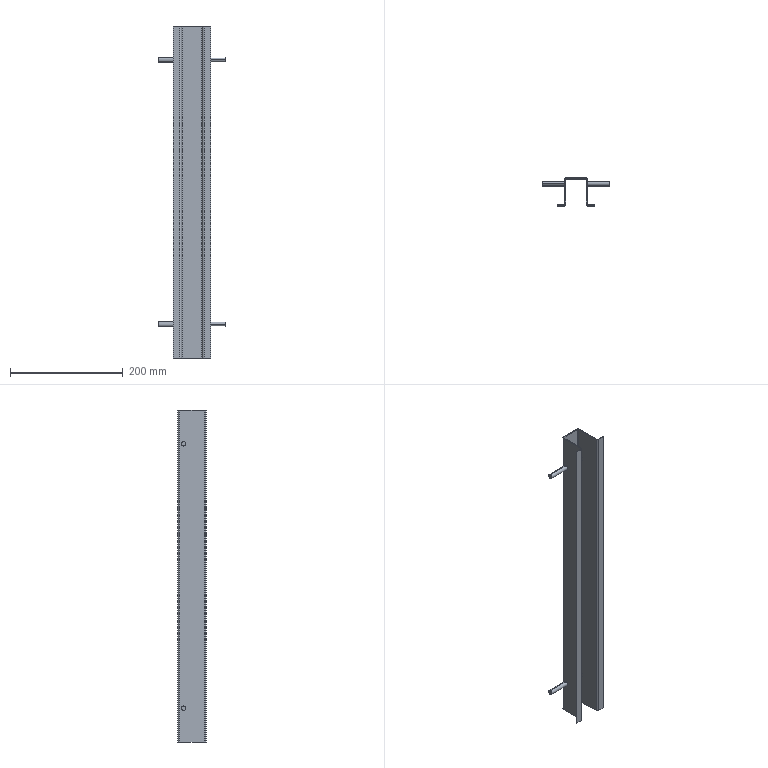Part | SolidWorks | features ICE 2, EdgeFlange 1, FlatPattern 1, SMBaseFlange 1, SheetMetal 1 | 1 solid | 50 faces | box 120 x 50 x 590 mm | volume 149764 mm3 | plane 34 | cylinder 16 | commonest cylinder face diameters 8 x8 3 x4 6 x4
STEP:
#1=CARTESIAN_POINT('',(-58.139,-0.4097,534.));
#2=VERTEX_POINT('',#1);
#3=CARTESIAN_POINT('',(-58.139,-0.4097,526.));
#4=VERTEX_POINT('',#3);
#5=CARTESIAN_POINT('',(-58.139,-0.4097,530.));
#6=DIRECTION('',(-1.,0.,0.));
#7=DIRECTION('',(0.,0.,1.));
#8=AXIS2_PLACEMENT_3D('',#5,#6,#7);
#9=CIRCLE('',#8,4.);
#10=EDGE_CURVE('',#2,#4,#9,.T.);
#11=ORIENTED_EDGE('',*,*,#10,.F.);
#12=CARTESIAN_POINT('',(-18.139,-0.4097,534.));
#13=VERTEX_POINT('',#12);
#14=CARTESIAN_POINT('',(-58.139,-0.4097,534.));
#15=DIRECTION('',(1.,0.,0.));
#16=VECTOR('',#15,1000.);
#17=LINE('',#14,#16);
#18=EDGE_CURVE('',#2,#13,#17,.T.);
#19=ORIENTED_EDGE('',*,*,#18,.T.);
#20=CARTESIAN_POINT('',(-18.139,-0.4097,526.));
#21=VERTEX_POINT('',#20);
#22=CARTESIAN_POINT('',(-18.139,-0.4097,530.));
#23=DIRECTION('',(-1.,0.,0.));
#24=DIRECTION('',(0.,0.,1.));
#25=AXIS2_PLACEMENT_3D('',#22,#23,#24);
#26=CIRCLE('',#25,4.);
#27=EDGE_CURVE('',#13,#21,#26,.T.);
#28=ORIENTED_EDGE('',*,*,#27,.T.);
#29=CARTESIAN_POINT('',(-58.139,-0.4097,526.));
#30=DIRECTION('',(1.,0.,0.));
#31=VECTOR('',#30,1000.);
#32=LINE('',#29,#31);
#33=EDGE_CURVE('',#4,#21,#32,.T.);
#34=ORIENTED_EDGE('',*,*,#33,.F.);
#35=EDGE_LOOP('',(#11,#19,#28,#34));
#36=FACE_OUTER_BOUND('',#35,.T.);
#37=CARTESIAN_POINT('',(-58.139,-0.4097,530.));
#38=DIRECTION('',(1.,0.,0.));
#39=DIRECTION('',(0.,0.,-1.));
#40=AXIS2_PLACEMENT_3D('',#37,#38,#39);
#41=CYLINDRICAL_SURFACE('',#40,4.);
#42=ADVANCED_FACE('',(#36),#41,.T.);
#43=CARTESIAN_POINT('',(-58.139,-0.4097,64.));
#44=VERTEX_POINT('',#43);
#45=CARTESIAN_POINT('',(-58.139,-0.4097,56.));
#46=VERTEX_POINT('',#45);
#47=CARTESIAN_POINT('',(-58.139,-0.4097,60.));
#48=DIRECTION('',(-1.,0.,0.));
#49=DIRECTION('',(0.,0.,1.));
#50=AXIS2_PLACEMENT_3D('',#47,#48,#49);
#51=CIRCLE('',#50,4.);
#52=EDGE_CURVE('',#44,#46,#51,.T.);
#53=ORIENTED_EDGE('',*,*,#52,.F.);
#54=CARTESIAN_POINT('',(-18.139,-0.4097,64.));
#55=VERTEX_POINT('',#54);
#56=CARTESIAN_POINT('',(-58.139,-0.4097,64.));
#57=DIRECTION('',(1.,0.,0.));
#58=VECTOR('',#57,1000.);
#59=LINE('',#56,#58);
#60=EDGE_CURVE('',#44,#55,#59,.T.);
#61=ORIENTED_EDGE('',*,*,#60,.T.);
#62=CARTESIAN_POINT('',(-18.139,-0.4097,56.));
#63=VERTEX_POINT('',#62);
#64=CARTESIAN_POINT('',(-18.139,-0.4097,60.));
#65=DIRECTION('',(-1.,0.,0.));
#66=DIRECTION('',(0.,0.,1.));
#67=AXIS2_PLACEMENT_3D('',#64,#65,#66);
#68=CIRCLE('',#67,4.);
#69=EDGE_CURVE('',#55,#63,#68,.T.);
#70=ORIENTED_EDGE('',*,*,#69,.T.);
#71=CARTESIAN_POINT('',(-58.139,-0.4097,56.));
#72=DIRECTION('',(1.,0.,0.));
#73=VECTOR('',#72,1000.);
#74=LINE('',#71,#73);
#75=EDGE_CURVE('',#46,#63,#74,.T.);
#76=ORIENTED_EDGE('',*,*,#75,.F.);
#77=EDGE_LOOP('',(#53,#61,#70,#76));
#78=FACE_OUTER_BOUND('',#77,.T.);
#79=CARTESIAN_POINT('',(-58.139,-0.4097,60.));
#80=DIRECTION('',(1.,0.,0.));
#81=DIRECTION('',(0.,0.,-1.));
#82=AXIS2_PLACEMENT_3D('',#79,#80,#81);
#83=CYLINDRICAL_SURFACE('',#82,4.);
#84=ADVANCED_FACE('',(#78),#83,.T.);
#85=CARTESIAN_POINT('',(61.861,3.59,60.));
#86=VERTEX_POINT('',#85);
#87=CARTESIAN_POINT('',(61.861,-4.41,60.));
#88=VERTEX_POINT('',#87);
#89=CARTESIAN_POINT('',(61.861,-0.4097,60.));
#90=DIRECTION('',(1.,0.,0.));
#91=DIRECTION('',(0.,1.,0.));
#92=AXIS2_PLACEMENT_3D('',#89,#90,#91);
#93=CIRCLE('',#92,4.);
#94=EDGE_CURVE('',#86,#88,#93,.T.);
#95=ORIENTED_EDGE('',*,*,#94,.F.);
#96=CARTESIAN_POINT('',(21.861,3.59,60.));
#97=VERTEX_POINT('',#96);
#98=CARTESIAN_POINT('',(61.861,3.59,60.));
#99=DIRECTION('',(-1.,0.,0.));
#100=VECTOR('',#99,1000.);
#101=LINE('',#98,#100);
#102=EDGE_CURVE('',#86,#97,#101,.T.);
#103=ORIENTED_EDGE('',*,*,#102,.T.);
#104=CARTESIAN_POINT('',(21.861,-4.41,60.));
#105=VERTEX_POINT('',#104);
#106=CARTESIAN_POINT('',(21.861,-0.4097,60.));
#107=DIRECTION('',(1.,0.,0.));
#108=DIRECTION('',(0.,1.,0.));
#109=AXIS2_PLACEMENT_3D('',#106,#107,#108);
#110=CIRCLE('',#109,4.);
#111=EDGE_CURVE('',#97,#105,#110,.T.);
#112=ORIENTED_EDGE('',*,*,#111,.T.);
#113=CARTESIAN_POINT('',(61.861,-4.41,60.));
#114=DIRECTION('',(-1.,0.,0.));
#115=VECTOR('',#114,1000.);
#116=LINE('',#113,#115);
#117=EDGE_CURVE('',#88,#105,#116,.T.);
#118=ORIENTED_EDGE('',*,*,#117,.F.);
#119=EDGE_LOOP('',(#95,#103,#112,#118));
#120=FACE_OUTER_BOUND('',#119,.T.);
#121=CARTESIAN_POINT('',(61.861,-0.4097,60.));
#122=DIRECTION('',(-1.,0.,0.));
#123=DIRECTION('',(0.,-1.,0.));
#124=AXIS2_PLACEMENT_3D('',#121,#122,#123);
#125=CYLINDRICAL_SURFACE('',#124,4.);
#126=ADVANCED_FACE('',(#120),#125,.T.);
#127=CARTESIAN_POINT('',(61.861,3.59,530.));
#128=VERTEX_POINT('',#127);
#129=CARTESIAN_POINT('',(61.861,-4.41,530.));
#130=VERTEX_POINT('',#129);
#131=CARTESIAN_POINT('',(61.861,-0.4097,530.));
#132=DIRECTION('',(1.,0.,0.));
#133=DIRECTION('',(0.,1.,0.));
#134=AXIS2_PLACEMENT_3D('',#131,#132,#133);
#135=CIRCLE('',#134,4.);
#136=EDGE_CURVE('',#128,#130,#135,.T.);
#137=ORIENTED_EDGE('',*,*,#136,.F.);
#138=CARTESIAN_POINT('',(21.861,3.59,530.));
#139=VERTEX_POINT('',#138);
#140=CARTESIAN_POINT('',(61.861,3.59,530.));
#141=DIRECTION('',(-1.,0.,0.));
#142=VECTOR('',#141,1000.);
#143=LINE('',#140,#142);
#144=EDGE_CURVE('',#128,#139,#143,.T.);
#145=ORIENTED_EDGE('',*,*,#144,.T.);
#146=CARTESIAN_POINT('',(21.861,-4.41,530.));
#147=VERTEX_POINT('',#146);
#148=CARTESIAN_POINT('',(21.861,-0.4097,530.));
#149=DIRECTION('',(1.,0.,0.));
#150=DIRECTION('',(0.,1.,0.));
#151=AXIS2_PLACEMENT_3D('',#148,#149,#150);
#152=CIRCLE('',#151,4.);
#153=EDGE_CURVE('',#139,#147,#152,.T.);
#154=ORIENTED_EDGE('',*,*,#153,.T.);
#155=CARTESIAN_POINT('',(61.861,-4.41,530.));
#156=DIRECTION('',(-1.,0.,0.));
#157=VECTOR('',#156,1000.);
#158=LINE('',#155,#157);
#159=EDGE_CURVE('',#130,#147,#158,.T.);
#160=ORIENTED_EDGE('',*,*,#159,.F.);
#161=EDGE_LOOP('',(#137,#145,#154,#160));
#162=FACE_OUTER_BOUND('',#161,.T.);
#163=CARTESIAN_POINT('',(61.861,-0.4097,530.));
#164=DIRECTION('',(-1.,0.,0.));
#165=DIRECTION('',(0.,-1.,0.));
#166=AXIS2_PLACEMENT_3D('',#163,#164,#165);
#167=CYLINDRICAL_SURFACE('',#166,4.);
#168=ADVANCED_FACE('',(#162),#167,.T.);
#169=CARTESIAN_POINT('',(-18.139,-0.4097,60.));
#170=DIRECTION('',(-1.,0.,0.));
#171=DIRECTION('',(0.,0.,1.));
#172=AXIS2_PLACEMENT_3D('',#169,#170,#171);
#173=CIRCLE('',#172,4.);
#174=EDGE_CURVE('',#63,#55,#173,.T.);
#175=ORIENTED_EDGE('',*,*,#174,.F.);
#176=ORIENTED_EDGE('',*,*,#69,.F.);
#177=EDGE_LOOP('',(#175,#176));
#178=FACE_BOUND('',#177,.T.);
#179=CARTESIAN_POINT('',(-18.139,-37.41,0.));
#180=VERTEX_POINT('',#179);
#181=CARTESIAN_POINT('',(-18.139,6.59,0.));
#182=VERTEX_POINT('',#181);
#183=CARTESIAN_POINT('',(-18.139,-40.41,0.));
#184=DIRECTION('',(0.,1.,0.));
#185=VECTOR('',#184,1000.);
#186=LINE('',#183,#185);
#187=EDGE_CURVE('',#180,#182,#186,.T.);
#188=ORIENTED_EDGE('',*,*,#187,.F.);
#189=CARTESIAN_POINT('',(-18.139,-37.41,590.));
#190=VERTEX_POINT('',#189);
#191=CARTESIAN_POINT('',(-18.139,-37.41,590.));
#192=DIRECTION('',(0.,0.,-1.));
#193=VECTOR('',#192,1000.);
#194=LINE('',#191,#193);
#195=EDGE_CURVE('',#190,#180,#194,.T.);
#196=ORIENTED_EDGE('',*,*,#195,.F.);
#197=CARTESIAN_POINT('',(-18.139,6.59,590.));
#198=VERTEX_POINT('',#197);
#199=CARTESIAN_POINT('',(-18.139,-40.41,590.));
#200=DIRECTION('',(0.,1.,0.));
#201=VECTOR('',#200,1000.);
#202=LINE('',#199,#201);
#203=EDGE_CURVE('',#190,#198,#202,.T.);
#204=ORIENTED_EDGE('',*,*,#203,.T.);
#205=CARTESIAN_POINT('',(-18.139,6.59,590.));
#206=DIRECTION('',(0.,0.,-1.));
#207=VECTOR('',#206,1000.);
#208=LINE('',#205,#207);
#209=EDGE_CURVE('',#198,#182,#208,.T.);
#210=ORIENTED_EDGE('',*,*,#209,.T.);
#211=EDGE_LOOP('',(#188,#196,#204,#210));
#212=FACE_OUTER_BOUND('',#211,.T.);
#213=CARTESIAN_POINT('',(-18.139,-0.4097,530.));
#214=DIRECTION('',(-1.,0.,0.));
#215=DIRECTION('',(0.,0.,1.));
#216=AXIS2_PLACEMENT_3D('',#213,#214,#215);
#217=CIRCLE('',#216,4.);
#218=EDGE_CURVE('',#21,#13,#217,.T.);
#219=ORIENTED_EDGE('',*,*,#218,.F.);
#220=ORIENTED_EDGE('',*,*,#27,.F.);
#221=EDGE_LOOP('',(#219,#220));
#222=FACE_BOUND('',#221,.T.);
#223=CARTESIAN_POINT('',(-18.139,-40.41,590.));
#224=DIRECTION('',(-1.,0.,0.));
#225=DIRECTION('',(0.,0.,1.));
#226=AXIS2_PLACEMENT_3D('',#223,#224,#225);
#227=PLANE('',#226);
#228=ADVANCED_FACE('',(#178,#212,#222),#227,.T.);
#229=CARTESIAN_POINT('',(21.861,-0.4097,530.));
#230=DIRECTION('',(1.,0.,0.));
#231=DIRECTION('',(0.,1.,0.));
#232=AXIS2_PLACEMENT_3D('',#229,#230,#231);
#233=CIRCLE('',#232,4.);
#234=EDGE_CURVE('',#147,#139,#233,.T.);
#235=ORIENTED_EDGE('',*,*,#234,.F.);
#236=ORIENTED_EDGE('',*,*,#153,.F.);
#237=EDGE_LOOP('',(#235,#236));
#238=FACE_BOUND('',#237,.T.);
#239=CARTESIAN_POINT('',(21.861,6.59,590.));
#240=VERTEX_POINT('',#239);
#241=CARTESIAN_POINT('',(21.861,-37.41,590.));
#242=VERTEX_POINT('',#241);
#243=CARTESIAN_POINT('',(21.861,9.59,590.));
#244=DIRECTION('',(0.,-1.,0.));
#245=VECTOR('',#244,1000.);
#246=LINE('',#243,#245);
#247=EDGE_CURVE('',#240,#242,#246,.T.);
#248=ORIENTED_EDGE('',*,*,#247,.T.);
#249=CARTESIAN_POINT('',(21.861,-37.41,0.));
#250=VERTEX_POINT('',#249);
#251=CARTESIAN_POINT('',(21.861,-37.41,0.));
#252=DIRECTION('',(0.,0.,1.));
#253=VECTOR('',#252,1000.);
#254=LINE('',#251,#253);
#255=EDGE_CURVE('',#250,#242,#254,.T.);
#256=ORIENTED_EDGE('',*,*,#255,.F.);
#257=CARTESIAN_POINT('',(21.861,6.59,0.));
#258=VERTEX_POINT('',#257);
#259=CARTESIAN_POINT('',(21.861,9.59,0.));
#260=DIRECTION('',(0.,-1.,0.));
#261=VECTOR('',#260,1000.);
#262=LINE('',#259,#261);
#263=EDGE_CURVE('',#258,#250,#262,.T.);
#264=ORIENTED_EDGE('',*,*,#263,.F.);
#265=CARTESIAN_POINT('',(21.861,6.59,590.));
#266=DIRECTION('',(0.,0.,-1.));
#267=VECTOR('',#266,1000.);
#268=LINE('',#265,#267);
#269=EDGE_CURVE('',#240,#258,#268,.T.);
#270=ORIENTED_EDGE('',*,*,#269,.F.);
#271=EDGE_LOOP('',(#248,#256,#264,#270));
#272=FACE_OUTER_BOUND('',#271,.T.);
#273=CARTESIAN_POINT('',(21.861,-0.4097,60.));
#274=DIRECTION('',(1.,0.,0.));
#275=DIRECTION('',(0.,1.,0.));
#276=AXIS2_PLACEMENT_3D('',#273,#274,#275);
#277=CIRCLE('',#276,4.);
#278=EDGE_CURVE('',#105,#97,#277,.T.);
#279=ORIENTED_EDGE('',*,*,#278,.F.);
#280=ORIENTED_EDGE('',*,*,#111,.F.);
#281=EDGE_LOOP('',(#279,#280));
#282=FACE_BOUND('',#281,.T.);
#283=CARTESIAN_POINT('',(21.861,9.59,590.));
#284=DIRECTION('',(1.,0.,0.));
#285=DIRECTION('',(0.,1.,0.));
#286=AXIS2_PLACEMENT_3D('',#283,#284,#285);
#287=PLANE('',#286);
#288=ADVANCED_FACE('',(#238,#272,#282),#287,.T.);
#289=CARTESIAN_POINT('',(-16.639,-37.41,590.));
#290=VERTEX_POINT('',#289);
#291=CARTESIAN_POINT('',(-16.639,-37.41,0.));
#292=VERTEX_POINT('',#291);
#293=CARTESIAN_POINT('',(-16.639,-37.41,590.));
#294=DIRECTION('',(0.,0.,-1.));
#295=VECTOR('',#294,1000.);
#296=LINE('',#293,#295);
#297=EDGE_CURVE('',#290,#292,#296,.T.);
#298=ORIENTED_EDGE('',*,*,#297,.T.);
#299=CARTESIAN_POINT('',(-16.639,6.59,0.));
#300=VERTEX_POINT('',#299);
#301=CARTESIAN_POINT('',(-16.639,-40.41,0.));
#302=DIRECTION('',(0.,1.,0.));
#303=VECTOR('',#302,1000.);
#304=LINE('',#301,#303);
#305=EDGE_CURVE('',#292,#300,#304,.T.);
#306=ORIENTED_EDGE('',*,*,#305,.T.);
#307=CARTESIAN_POINT('',(-16.639,6.59,590.));
#308=VERTEX_POINT('',#307);
#309=CARTESIAN_POINT('',(-16.639,6.59,590.));
#310=DIRECTION('',(0.,0.,-1.));
#311=VECTOR('',#310,1000.);
#312=LINE('',#309,#311);
#313=EDGE_CURVE('',#308,#300,#312,.T.);
#314=ORIENTED_EDGE('',*,*,#313,.F.);
#315=CARTESIAN_POINT('',(-16.639,-40.41,590.));
#316=DIRECTION('',(0.,1.,0.));
#317=VECTOR('',#316,1000.);
#318=LINE('',#315,#317);
#319=EDGE_CURVE('',#290,#308,#318,.T.);
#320=ORIENTED_EDGE('',*,*,#319,.F.);
#321=EDGE_LOOP('',(#298,#306,#314,#320));
#322=FACE_OUTER_BOUND('',#321,.T.);
#323=CARTESIAN_POINT('',(-16.639,-40.41,590.));
#324=DIRECTION('',(-1.,0.,0.));
#325=DIRECTION('',(0.,0.,1.));
#326=AXIS2_PLACEMENT_3D('',#323,#324,#325);
#327=PLANE('',#326);
#328=ADVANCED_FACE('',(#322),#327,.F.);
#329=ORIENTED_EDGE('',*,*,#203,.F.);
#330=CARTESIAN_POINT('',(-18.139,-37.41,590.));
#331=DIRECTION('',(1.,0.,0.));
#332=VECTOR('',#331,1000.);
#333=LINE('',#330,#332);
#334=EDGE_CURVE('',#190,#290,#333,.T.);
#335=ORIENTED_EDGE('',*,*,#334,.T.);
#336=ORIENTED_EDGE('',*,*,#319,.T.);
#337=CARTESIAN_POINT('',(-16.639,6.59,590.));
#338=DIRECTION('',(-1.,0.,0.));
#339=VECTOR('',#338,1000.);
#340=LINE('',#337,#339);
#341=EDGE_CURVE('',#308,#198,#340,.T.);
#342=ORIENTED_EDGE('',*,*,#341,.T.);
#343=EDGE_LOOP('',(#329,#335,#336,#342));
#344=FACE_OUTER_BOUND('',#343,.T.);
#345=CARTESIAN_POINT('',(18.861,6.59,590.));
#346=DIRECTION('',(0.,0.,1.));
#347=DIRECTION('',(1.,0.,0.));
#348=AXIS2_PLACEMENT_3D('',#345,#346,#347);
#349=PLANE('',#348);
#350=ADVANCED_FACE('',(#344),#349,.T.);
#351=CARTESIAN_POINT('',(20.361,-37.41,0.));
#352=VERTEX_POINT('',#351);
#353=CARTESIAN_POINT('',(20.361,-37.41,590.));
#354=VERTEX_POINT('',#353);
#355=CARTESIAN_POINT('',(20.361,-37.41,0.));
#356=DIRECTION('',(0.,0.,1.));
#357=VECTOR('',#356,1000.);
#358=LINE('',#355,#357);
#359=EDGE_CURVE('',#352,#354,#358,.T.);
#360=ORIENTED_EDGE('',*,*,#359,.T.);
#361=CARTESIAN_POINT('',(20.361,6.59,590.));
#362=VERTEX_POINT('',#361);
#363=CARTESIAN_POINT('',(20.361,9.59,590.));
#364=DIRECTION('',(0.,-1.,0.));
#365=VECTOR('',#364,1000.);
#366=LINE('',#363,#365);
#367=EDGE_CURVE('',#362,#354,#366,.T.);
#368=ORIENTED_EDGE('',*,*,#367,.F.);
#369=CARTESIAN_POINT('',(20.361,6.59,0.));
#370=VERTEX_POINT('',#369);
#371=CARTESIAN_POINT('',(20.361,6.59,590.));
#372=DIRECTION('',(0.,0.,-1.));
#373=VECTOR('',#372,1000.);
#374=LINE('',#371,#373);
#375=EDGE_CURVE('',#362,#370,#374,.T.);
#376=ORIENTED_EDGE('',*,*,#375,.T.);
#377=CARTESIAN_POINT('',(20.361,9.59,0.));
#378=DIRECTION('',(0.,-1.,0.));
#379=VECTOR('',#378,1000.);
#380=LINE('',#377,#379);
#381=EDGE_CURVE('',#370,#352,#380,.T.);
#382=ORIENTED_EDGE('',*,*,#381,.T.);
#383=EDGE_LOOP('',(#360,#368,#376,#382));
#384=FACE_OUTER_BOUND('',#383,.T.);
#385=CARTESIAN_POINT('',(20.361,9.59,590.));
#386=DIRECTION('',(1.,0.,0.));
#387=DIRECTION('',(0.,1.,0.));
#388=AXIS2_PLACEMENT_3D('',#385,#386,#387);
#389=PLANE('',#388);
#390=ADVANCED_FACE('',(#384),#389,.F.);
#391=CARTESIAN_POINT('',(21.861,-37.41,0.));
#392=DIRECTION('',(-1.,0.,0.));
#393=VECTOR('',#392,1000.);
#394=LINE('',#391,#393);
#395=EDGE_CURVE('',#250,#352,#394,.T.);
#396=ORIENTED_EDGE('',*,*,#395,.T.);
#397=ORIENTED_EDGE('',*,*,#381,.F.);
#398=CARTESIAN_POINT('',(20.361,6.59,0.));
#399=DIRECTION('',(1.,0.,0.));
#400=VECTOR('',#399,1000.);
#401=LINE('',#398,#400);
#402=EDGE_CURVE('',#370,#258,#401,.T.);
#403=ORIENTED_EDGE('',*,*,#402,.T.);
#404=ORIENTED_EDGE('',*,*,#263,.T.);
#405=EDGE_LOOP('',(#396,#397,#403,#404));
#406=FACE_OUTER_BOUND('',#405,.T.);
#407=CARTESIAN_POINT('',(18.861,6.59,0.));
#408=DIRECTION('',(0.,0.,1.));
#409=DIRECTION('',(1.,0.,0.));
#410=AXIS2_PLACEMENT_3D('',#407,#408,#409);
#411=PLANE('',#410);
#412=ADVANCED_FACE('',(#406),#411,.F.);
#413=CARTESIAN_POINT('',(-15.139,9.59,590.));
#414=VERTEX_POINT('',#413);
#415=CARTESIAN_POINT('',(-15.139,8.09,590.));
#416=VERTEX_POINT('',#415);
#417=CARTESIAN_POINT('',(-15.139,9.59,590.));
#418=DIRECTION('',(0.,-1.,0.));
#419=VECTOR('',#418,1000.);
#420=LINE('',#417,#419);
#421=EDGE_CURVE('',#414,#416,#420,.T.);
#422=ORIENTED_EDGE('',*,*,#421,.F.);
#423=CARTESIAN_POINT('',(-15.139,6.59,590.));
#424=DIRECTION('',(0.,0.,-1.));
#425=DIRECTION('',(1.,0.,0.));
#426=AXIS2_PLACEMENT_3D('',#423,#424,#425);
#427=CIRCLE('',#426,3.);
#428=EDGE_CURVE('',#198,#414,#427,.T.);
#429=ORIENTED_EDGE('',*,*,#428,.F.);
#430=ORIENTED_EDGE('',*,*,#341,.F.);
#431=CARTESIAN_POINT('',(-15.139,6.59,590.));
#432=DIRECTION('',(0.,0.,-1.));
#433=DIRECTION('',(1.,0.,0.));
#434=AXIS2_PLACEMENT_3D('',#431,#432,#433);
#435=CIRCLE('',#434,1.5);
#436=EDGE_CURVE('',#308,#416,#435,.T.);
#437=ORIENTED_EDGE('',*,*,#436,.T.);
#438=EDGE_LOOP('',(#422,#429,#430,#437));
#439=FACE_OUTER_BOUND('',#438,.T.);
#440=CARTESIAN_POINT('',(-15.139,9.59,590.));
#441=DIRECTION('',(0.,0.,1.));
#442=DIRECTION('',(1.,0.,0.));
#443=AXIS2_PLACEMENT_3D('',#440,#441,#442);
#444=PLANE('',#443);
#445=ADVANCED_FACE('',(#439),#444,.T.);
#446=CARTESIAN_POINT('',(18.861,9.59,590.));
#447=VERTEX_POINT('',#446);
#448=CARTESIAN_POINT('',(-18.139,9.59,590.));
#449=DIRECTION('',(1.,0.,0.));
#450=VECTOR('',#449,1000.);
#451=LINE('',#448,#450);
#452=EDGE_CURVE('',#414,#447,#451,.T.);
#453=ORIENTED_EDGE('',*,*,#452,.F.);
#454=ORIENTED_EDGE('',*,*,#421,.T.);
#455=CARTESIAN_POINT('',(18.861,8.09,590.));
#456=VERTEX_POINT('',#455);
#457=CARTESIAN_POINT('',(-18.139,8.09,590.));
#458=DIRECTION('',(1.,0.,0.));
#459=VECTOR('',#458,1000.);
#460=LINE('',#457,#459);
#461=EDGE_CURVE('',#416,#456,#460,.T.);
#462=ORIENTED_EDGE('',*,*,#461,.T.);
#463=CARTESIAN_POINT('',(18.861,8.09,590.));
#464=DIRECTION('',(0.,1.,0.));
#465=VECTOR('',#464,1000.);
#466=LINE('',#463,#465);
#467=EDGE_CURVE('',#456,#447,#466,.T.);
#468=ORIENTED_EDGE('',*,*,#467,.T.);
#469=EDGE_LOOP('',(#453,#454,#462,#468));
#470=FACE_OUTER_BOUND('',#469,.T.);
#471=CARTESIAN_POINT('',(-16.639,6.59,590.));
#472=DIRECTION('',(0.,0.,1.));
#473=DIRECTION('',(1.,0.,0.));
#474=AXIS2_PLACEMENT_3D('',#471,#472,#473);
#475=PLANE('',#474);
#476=ADVANCED_FACE('',(#470),#475,.T.);
#477=CARTESIAN_POINT('',(-18.139,6.59,0.));
#478=DIRECTION('',(1.,0.,0.));
#479=VECTOR('',#478,1000.);
#480=LINE('',#477,#479);
#481=EDGE_CURVE('',#182,#300,#480,.T.);
#482=ORIENTED_EDGE('',*,*,#481,.F.);
#483=CARTESIAN_POINT('',(-15.139,9.59,0.));
#484=VERTEX_POINT('',#483);
#485=CARTESIAN_POINT('',(-15.139,6.59,0.));
#486=DIRECTION('',(0.,0.,-1.));
#487=DIRECTION('',(1.,0.,0.));
#488=AXIS2_PLACEMENT_3D('',#485,#486,#487);
#489=CIRCLE('',#488,3.);
#490=EDGE_CURVE('',#182,#484,#489,.T.);
#491=ORIENTED_EDGE('',*,*,#490,.T.);
#492=CARTESIAN_POINT('',(-15.139,8.09,0.));
#493=VERTEX_POINT('',#492);
#494=CARTESIAN_POINT('',(-15.139,8.09,0.));
#495=DIRECTION('',(0.,1.,0.));
#496=VECTOR('',#495,1000.);
#497=LINE('',#494,#496);
#498=EDGE_CURVE('',#493,#484,#497,.T.);
#499=ORIENTED_EDGE('',*,*,#498,.F.);
#500=CARTESIAN_POINT('',(-15.139,6.59,0.));
#501=DIRECTION('',(0.,0.,-1.));
#502=DIRECTION('',(1.,0.,0.));
#503=AXIS2_PLACEMENT_3D('',#500,#501,#502);
#504=CIRCLE('',#503,1.5);
#505=EDGE_CURVE('',#300,#493,#504,.T.);
#506=ORIENTED_EDGE('',*,*,#505,.F.);
#507=EDGE_LOOP('',(#482,#491,#499,#506));
#508=FACE_OUTER_BOUND('',#507,.T.);
#509=CARTESIAN_POINT('',(-18.139,6.59,0.));
#510=DIRECTION('',(0.,0.,-1.));
#511=DIRECTION('',(-1.,0.,0.));
#512=AXIS2_PLACEMENT_3D('',#509,#510,#511);
#513=PLANE('',#512);
#514=ADVANCED_FACE('',(#508),#513,.T.);
#515=CARTESIAN_POINT('',(-18.139,-37.41,0.));
#516=DIRECTION('',(1.,0.,0.));
#517=VECTOR('',#516,1000.);
#518=LINE('',#515,#517);
#519=EDGE_CURVE('',#180,#292,#518,.T.);
#520=ORIENTED_EDGE('',*,*,#519,.F.);
#521=ORIENTED_EDGE('',*,*,#187,.T.);
#522=ORIENTED_EDGE('',*,*,#481,.T.);
#523=ORIENTED_EDGE('',*,*,#305,.F.);
#524=EDGE_LOOP('',(#520,#521,#522,#523));
#525=FACE_OUTER_BOUND('',#524,.T.);
#526=CARTESIAN_POINT('',(-15.139,8.09,0.));
#527=DIRECTION('',(0.,0.,-1.));
#528=DIRECTION('',(-1.,0.,0.));
#529=AXIS2_PLACEMENT_3D('',#526,#527,#528);
#530=PLANE('',#529);
#531=ADVANCED_FACE('',(#525),#530,.T.);
#532=CARTESIAN_POINT('',(21.861,6.59,590.));
#533=DIRECTION('',(-1.,0.,0.));
#534=VECTOR('',#533,1000.);
#535=LINE('',#532,#534);
#536=EDGE_CURVE('',#240,#362,#535,.T.);
#537=ORIENTED_EDGE('',*,*,#536,.F.);
#538=CARTESIAN_POINT('',(18.861,6.59,590.));
#539=DIRECTION('',(0.,0.,-1.));
#540=DIRECTION('',(1.,0.,0.));
#541=AXIS2_PLACEMENT_3D('',#538,#539,#540);
#542=CIRCLE('',#541,3.);
#543=EDGE_CURVE('',#447,#240,#542,.T.);
#544=ORIENTED_EDGE('',*,*,#543,.F.);
#545=ORIENTED_EDGE('',*,*,#467,.F.);
#546=CARTESIAN_POINT('',(18.861,6.59,590.));
#547=DIRECTION('',(0.,0.,-1.));
#548=DIRECTION('',(1.,0.,0.));
#549=AXIS2_PLACEMENT_3D('',#546,#547,#548);
#550=CIRCLE('',#549,1.5);
#551=EDGE_CURVE('',#456,#362,#550,.T.);
#552=ORIENTED_EDGE('',*,*,#551,.T.);
#553=EDGE_LOOP('',(#537,#544,#545,#552));
#554=FACE_OUTER_BOUND('',#553,.T.);
#555=CARTESIAN_POINT('',(21.861,6.59,590.));
#556=DIRECTION('',(0.,0.,1.));
#557=DIRECTION('',(1.,0.,0.));
#558=AXIS2_PLACEMENT_3D('',#555,#556,#557);
#559=PLANE('',#558);
#560=ADVANCED_FACE('',(#554),#559,.T.);
#561=CARTESIAN_POINT('',(21.861,-37.41,590.));
#562=DIRECTION('',(-1.,0.,0.));
#563=VECTOR('',#562,1000.);
#564=LINE('',#561,#563);
#565=EDGE_CURVE('',#242,#354,#564,.T.);
#566=ORIENTED_EDGE('',*,*,#565,.F.);
#567=ORIENTED_EDGE('',*,*,#247,.F.);
#568=ORIENTED_EDGE('',*,*,#536,.T.);
#569=ORIENTED_EDGE('',*,*,#367,.T.);
#570=EDGE_LOOP('',(#566,#567,#568,#569));
#571=FACE_OUTER_BOUND('',#570,.T.);
#572=CARTESIAN_POINT('',(18.861,8.09,590.));
#573=DIRECTION('',(0.,0.,1.));
#574=DIRECTION('',(1.,0.,0.));
#575=AXIS2_PLACEMENT_3D('',#572,#573,#574);
#576=PLANE('',#575);
#577=ADVANCED_FACE('',(#571),#576,.T.);
#578=CARTESIAN_POINT('',(18.861,9.59,0.));
#579=VERTEX_POINT('',#578);
#580=CARTESIAN_POINT('',(18.861,8.09,0.));
#581=VERTEX_POINT('',#580);
#582=CARTESIAN_POINT('',(18.861,9.59,0.));
#583=DIRECTION('',(0.,-1.,0.));
#584=VECTOR('',#583,1000.);
#585=LINE('',#582,#584);
#586=EDGE_CURVE('',#579,#581,#585,.T.);
#587=ORIENTED_EDGE('',*,*,#586,.F.);
#588=CARTESIAN_POINT('',(18.861,6.59,0.));
#589=DIRECTION('',(0.,0.,-1.));
#590=DIRECTION('',(1.,0.,0.));
#591=AXIS2_PLACEMENT_3D('',#588,#589,#590);
#592=CIRCLE('',#591,3.);
#593=EDGE_CURVE('',#579,#258,#592,.T.);
#594=ORIENTED_EDGE('',*,*,#593,.T.);
#595=ORIENTED_EDGE('',*,*,#402,.F.);
#596=CARTESIAN_POINT('',(18.861,6.59,0.));
#597=DIRECTION('',(0.,0.,-1.));
#598=DIRECTION('',(1.,0.,0.));
#599=AXIS2_PLACEMENT_3D('',#596,#597,#598);
#600=CIRCLE('',#599,1.5);
#601=EDGE_CURVE('',#581,#370,#600,.T.);
#602=ORIENTED_EDGE('',*,*,#601,.F.);
#603=EDGE_LOOP('',(#587,#594,#595,#602));
#604=FACE_OUTER_BOUND('',#603,.T.);
#605=CARTESIAN_POINT('',(18.861,9.59,0.));
#606=DIRECTION('',(0.,0.,-1.));
#607=DIRECTION('',(-1.,0.,0.));
#608=AXIS2_PLACEMENT_3D('',#605,#606,#607);
#609=PLANE('',#608);
#610=ADVANCED_FACE('',(#604),#609,.T.);
#611=CARTESIAN_POINT('',(-18.139,9.59,0.));
#612=DIRECTION('',(1.,0.,0.));
#613=VECTOR('',#612,1000.);
#614=LINE('',#611,#613);
#615=EDGE_CURVE('',#484,#579,#614,.T.);
#616=ORIENTED_EDGE('',*,*,#615,.T.);
#617=ORIENTED_EDGE('',*,*,#586,.T.);
#618=CARTESIAN_POINT('',(-18.139,8.09,0.));
#619=DIRECTION('',(1.,0.,0.));
#620=VECTOR('',#619,1000.);
#621=LINE('',#618,#620);
#622=EDGE_CURVE('',#493,#581,#621,.T.);
#623=ORIENTED_EDGE('',*,*,#622,.F.);
#624=ORIENTED_EDGE('',*,*,#498,.T.);
#625=EDGE_LOOP('',(#616,#617,#623,#624));
#626=FACE_OUTER_BOUND('',#625,.T.);
#627=CARTESIAN_POINT('',(20.361,6.59,0.));
#628=DIRECTION('',(0.,0.,-1.));
#629=DIRECTION('',(-1.,0.,0.));
#630=AXIS2_PLACEMENT_3D('',#627,#628,#629);
#631=PLANE('',#630);
#632=ADVANCED_FACE('',(#626),#631,.T.);
#633=ORIENTED_EDGE('',*,*,#593,.F.);
#634=CARTESIAN_POINT('',(18.861,9.59,590.));
#635=DIRECTION('',(0.,0.,-1.));
#636=VECTOR('',#635,1000.);
#637=LINE('',#634,#636);
#638=EDGE_CURVE('',#447,#579,#637,.T.);
#639=ORIENTED_EDGE('',*,*,#638,.F.);
#640=ORIENTED_EDGE('',*,*,#543,.T.);
#641=ORIENTED_EDGE('',*,*,#269,.T.);
#642=EDGE_LOOP('',(#633,#639,#640,#641));
#643=FACE_OUTER_BOUND('',#642,.T.);
#644=CARTESIAN_POINT('',(18.861,6.59,590.));
#645=DIRECTION('',(0.,0.,-1.));
#646=DIRECTION('',(-1.,0.,0.));
#647=AXIS2_PLACEMENT_3D('',#644,#645,#646);
#648=CYLINDRICAL_SURFACE('',#647,3.);
#649=ADVANCED_FACE('',(#643),#648,.T.);
#650=ORIENTED_EDGE('',*,*,#615,.F.);
#651=CARTESIAN_POINT('',(-15.139,9.59,590.));
#652=DIRECTION('',(0.,0.,-1.));
#653=VECTOR('',#652,1000.);
#654=LINE('',#651,#653);
#655=EDGE_CURVE('',#414,#484,#654,.T.);
#656=ORIENTED_EDGE('',*,*,#655,.F.);
#657=ORIENTED_EDGE('',*,*,#452,.T.);
#658=ORIENTED_EDGE('',*,*,#638,.T.);
#659=EDGE_LOOP('',(#650,#656,#657,#658));
#660=FACE_OUTER_BOUND('',#659,.T.);
#661=CARTESIAN_POINT('',(-18.139,9.59,590.));
#662=DIRECTION('',(0.,1.,0.));
#663=DIRECTION('',(0.,0.,1.));
#664=AXIS2_PLACEMENT_3D('',#661,#662,#663);
#665=PLANE('',#664);
#666=ADVANCED_FACE('',(#660),#665,.T.);
#667=ORIENTED_EDGE('',*,*,#490,.F.);
#668=ORIENTED_EDGE('',*,*,#209,.F.);
#669=ORIENTED_EDGE('',*,*,#428,.T.);
#670=ORIENTED_EDGE('',*,*,#655,.T.);
#671=EDGE_LOOP('',(#667,#668,#669,#670));
#672=FACE_OUTER_BOUND('',#671,.T.);
#673=CARTESIAN_POINT('',(-15.139,6.59,590.));
#674=DIRECTION('',(0.,0.,-1.));
#675=DIRECTION('',(-1.,0.,0.));
#676=AXIS2_PLACEMENT_3D('',#673,#674,#675);
#677=CYLINDRICAL_SURFACE('',#676,3.);
#678=ADVANCED_FACE('',(#672),#677,.T.);
#679=ORIENTED_EDGE('',*,*,#505,.T.);
#680=CARTESIAN_POINT('',(-15.139,8.09,590.));
#681=DIRECTION('',(0.,0.,-1.));
#682=VECTOR('',#681,1000.);
#683=LINE('',#680,#682);
#684=EDGE_CURVE('',#416,#493,#683,.T.);
#685=ORIENTED_EDGE('',*,*,#684,.F.);
#686=ORIENTED_EDGE('',*,*,#436,.F.);
#687=ORIENTED_EDGE('',*,*,#313,.T.);
#688=EDGE_LOOP('',(#679,#685,#686,#687));
#689=FACE_OUTER_BOUND('',#688,.T.);
#690=CARTESIAN_POINT('',(-15.139,6.59,590.));
#691=DIRECTION('',(0.,0.,-1.));
#692=DIRECTION('',(-1.,0.,0.));
#693=AXIS2_PLACEMENT_3D('',#690,#691,#692);
#694=CYLINDRICAL_SURFACE('',#693,1.5);
#695=ADVANCED_FACE('',(#689),#694,.F.);
#696=ORIENTED_EDGE('',*,*,#622,.T.);
#697=CARTESIAN_POINT('',(18.861,8.09,590.));
#698=DIRECTION('',(0.,0.,-1.));
#699=VECTOR('',#698,1000.);
#700=LINE('',#697,#699);
#701=EDGE_CURVE('',#456,#581,#700,.T.);
#702=ORIENTED_EDGE('',*,*,#701,.F.);
#703=ORIENTED_EDGE('',*,*,#461,.F.);
#704=ORIENTED_EDGE('',*,*,#684,.T.);
#705=EDGE_LOOP('',(#696,#702,#703,#704));
#706=FACE_OUTER_BOUND('',#705,.T.);
#707=CARTESIAN_POINT('',(-18.139,8.09,590.));
#708=DIRECTION('',(0.,1.,0.));
#709=DIRECTION('',(0.,0.,1.));
#710=AXIS2_PLACEMENT_3D('',#707,#708,#709);
#711=PLANE('',#710);
#712=ADVANCED_FACE('',(#706),#711,.F.);
#713=ORIENTED_EDGE('',*,*,#601,.T.);
#714=ORIENTED_EDGE('',*,*,#375,.F.);
#715=ORIENTED_EDGE('',*,*,#551,.F.);
#716=ORIENTED_EDGE('',*,*,#701,.T.);
#717=EDGE_LOOP('',(#713,#714,#715,#716));
#718=FACE_OUTER_BOUND('',#717,.T.);
#719=CARTESIAN_POINT('',(18.861,6.59,590.));
#720=DIRECTION('',(0.,0.,-1.));
#721=DIRECTION('',(-1.,0.,0.));
#722=AXIS2_PLACEMENT_3D('',#719,#720,#721);
#723=CYLINDRICAL_SURFACE('',#722,1.5);
#724=ADVANCED_FACE('',(#718),#723,.F.);
#725=CARTESIAN_POINT('',(23.361,-38.91,590.));
#726=VERTEX_POINT('',#725);
#727=CARTESIAN_POINT('',(23.361,-40.41,590.));
#728=VERTEX_POINT('',#727);
#729=CARTESIAN_POINT('',(23.361,-40.41,590.));
#730=DIRECTION('',(0.,-1.,0.));
#731=VECTOR('',#730,1000.);
#732=LINE('',#729,#731);
#733=EDGE_CURVE('',#726,#728,#732,.T.);
#734=ORIENTED_EDGE('',*,*,#733,.F.);
#735=CARTESIAN_POINT('',(23.361,-37.41,590.));
#736=DIRECTION('',(0.,0.,1.));
#737=DIRECTION('',(-1.,0.,0.));
#738=AXIS2_PLACEMENT_3D('',#735,#736,#737);
#739=CIRCLE('',#738,1.5);
#740=EDGE_CURVE('',#242,#726,#739,.T.);
#741=ORIENTED_EDGE('',*,*,#740,.F.);
#742=ORIENTED_EDGE('',*,*,#565,.T.);
#743=CARTESIAN_POINT('',(23.361,-37.41,590.));
#744=DIRECTION('',(0.,0.,1.));
#745=DIRECTION('',(-1.,0.,0.));
#746=AXIS2_PLACEMENT_3D('',#743,#744,#745);
#747=CIRCLE('',#746,3.);
#748=EDGE_CURVE('',#354,#728,#747,.T.);
#749=ORIENTED_EDGE('',*,*,#748,.T.);
#750=EDGE_LOOP('',(#734,#741,#742,#749));
#751=FACE_OUTER_BOUND('',#750,.T.);
#752=CARTESIAN_POINT('',(23.361,-37.41,590.));
#753=DIRECTION('',(0.,0.,1.));
#754=DIRECTION('',(1.,0.,0.));
#755=AXIS2_PLACEMENT_3D('',#752,#753,#754);
#756=PLANE('',#755);
#757=ADVANCED_FACE('',(#751),#756,.T.);
#758=CARTESIAN_POINT('',(23.361,-38.91,0.));
#759=VERTEX_POINT('',#758);
#760=CARTESIAN_POINT('',(23.361,-37.41,0.));
#761=DIRECTION('',(0.,0.,-1.));
#762=DIRECTION('',(-1.,0.,0.));
#763=AXIS2_PLACEMENT_3D('',#760,#761,#762);
#764=CIRCLE('',#763,1.5);
#765=EDGE_CURVE('',#759,#250,#764,.T.);
#766=ORIENTED_EDGE('',*,*,#765,.F.);
#767=CARTESIAN_POINT('',(23.361,-40.41,0.));
#768=VERTEX_POINT('',#767);
#769=CARTESIAN_POINT('',(23.361,-38.91,0.));
#770=DIRECTION('',(0.,-1.,0.));
#771=VECTOR('',#770,1000.);
#772=LINE('',#769,#771);
#773=EDGE_CURVE('',#759,#768,#772,.T.);
#774=ORIENTED_EDGE('',*,*,#773,.T.);
#775=CARTESIAN_POINT('',(23.361,-37.41,0.));
#776=DIRECTION('',(0.,0.,-1.));
#777=DIRECTION('',(-1.,0.,0.));
#778=AXIS2_PLACEMENT_3D('',#775,#776,#777);
#779=CIRCLE('',#778,3.);
#780=EDGE_CURVE('',#768,#352,#779,.T.);
#781=ORIENTED_EDGE('',*,*,#780,.T.);
#782=ORIENTED_EDGE('',*,*,#395,.F.);
#783=EDGE_LOOP('',(#766,#774,#781,#782));
#784=FACE_OUTER_BOUND('',#783,.T.);
#785=CARTESIAN_POINT('',(23.361,-37.41,0.));
#786=DIRECTION('',(0.,0.,1.));
#787=DIRECTION('',(1.,0.,0.));
#788=AXIS2_PLACEMENT_3D('',#785,#786,#787);
#789=PLANE('',#788);
#790=ADVANCED_FACE('',(#784),#789,.F.);
#791=ORIENTED_EDGE('',*,*,#359,.F.);
#792=ORIENTED_EDGE('',*,*,#780,.F.);
#793=CARTESIAN_POINT('',(23.361,-40.41,590.));
#794=DIRECTION('',(0.,0.,1.));
#795=VECTOR('',#794,1000.);
#796=LINE('',#793,#795);
#797=EDGE_CURVE('',#768,#728,#796,.T.);
#798=ORIENTED_EDGE('',*,*,#797,.T.);
#799=ORIENTED_EDGE('',*,*,#748,.F.);
#800=EDGE_LOOP('',(#791,#792,#798,#799));
#801=FACE_OUTER_BOUND('',#800,.T.);
#802=CARTESIAN_POINT('',(23.361,-37.41,0.));
#803=DIRECTION('',(0.,0.,-1.));
#804=DIRECTION('',(0.,-1.,0.));
#805=AXIS2_PLACEMENT_3D('',#802,#803,#804);
#806=CYLINDRICAL_SURFACE('',#805,3.);
#807=ADVANCED_FACE('',(#801),#806,.T.);
#808=ORIENTED_EDGE('',*,*,#255,.T.);
#809=ORIENTED_EDGE('',*,*,#740,.T.);
#810=CARTESIAN_POINT('',(23.361,-38.91,590.));
#811=DIRECTION('',(0.,0.,-1.));
#812=VECTOR('',#811,1000.);
#813=LINE('',#810,#812);
#814=EDGE_CURVE('',#726,#759,#813,.T.);
#815=ORIENTED_EDGE('',*,*,#814,.T.);
#816=ORIENTED_EDGE('',*,*,#765,.T.);
#817=EDGE_LOOP('',(#808,#809,#815,#816));
#818=FACE_OUTER_BOUND('',#817,.T.);
#819=CARTESIAN_POINT('',(23.361,-37.41,0.));
#820=DIRECTION('',(0.,0.,-1.));
#821=DIRECTION('',(0.,-1.,0.));
#822=AXIS2_PLACEMENT_3D('',#819,#820,#821);
#823=CYLINDRICAL_SURFACE('',#822,1.5);
#824=ADVANCED_FACE('',(#818),#823,.F.);
#825=ORIENTED_EDGE('',*,*,#773,.F.);
#826=CARTESIAN_POINT('',(35.361,-38.91,0.));
#827=VERTEX_POINT('',#826);
#828=CARTESIAN_POINT('',(35.361,-38.91,0.));
#829=DIRECTION('',(1.,0.,0.));
#830=VECTOR('',#829,1000.);
#831=LINE('',#828,#830);
#832=EDGE_CURVE('',#759,#827,#831,.T.);
#833=ORIENTED_EDGE('',*,*,#832,.T.);
#834=CARTESIAN_POINT('',(35.361,-40.41,0.));
#835=VERTEX_POINT('',#834);
#836=CARTESIAN_POINT('',(35.361,-40.41,0.));
#837=DIRECTION('',(0.,1.,0.));
#838=VECTOR('',#837,1000.);
#839=LINE('',#836,#838);
#840=EDGE_CURVE('',#835,#827,#839,.T.);
#841=ORIENTED_EDGE('',*,*,#840,.F.);
#842=CARTESIAN_POINT('',(0.,-40.41,0.));
#843=DIRECTION('',(1.,0.,0.));
#844=VECTOR('',#843,1000.);
#845=LINE('',#842,#844);
#846=EDGE_CURVE('',#768,#835,#845,.T.);
#847=ORIENTED_EDGE('',*,*,#846,.F.);
#848=EDGE_LOOP('',(#825,#833,#841,#847));
#849=FACE_OUTER_BOUND('',#848,.T.);
#850=CARTESIAN_POINT('',(35.361,-40.41,0.));
#851=DIRECTION('',(0.,0.,1.));
#852=DIRECTION('',(1.,0.,0.));
#853=AXIS2_PLACEMENT_3D('',#850,#851,#852);
#854=PLANE('',#853);
#855=ADVANCED_FACE('',(#849),#854,.F.);
#856=ORIENTED_EDGE('',*,*,#733,.T.);
#857=CARTESIAN_POINT('',(35.361,-40.41,590.));
#858=VERTEX_POINT('',#857);
#859=CARTESIAN_POINT('',(0.,-40.41,590.));
#860=DIRECTION('',(-1.,0.,0.));
#861=VECTOR('',#860,1000.);
#862=LINE('',#859,#861);
#863=EDGE_CURVE('',#858,#728,#862,.T.);
#864=ORIENTED_EDGE('',*,*,#863,.F.);
#865=CARTESIAN_POINT('',(35.361,-38.91,590.));
#866=VERTEX_POINT('',#865);
#867=CARTESIAN_POINT('',(35.361,-40.41,590.));
#868=DIRECTION('',(0.,1.,0.));
#869=VECTOR('',#868,1000.);
#870=LINE('',#867,#869);
#871=EDGE_CURVE('',#858,#866,#870,.T.);
#872=ORIENTED_EDGE('',*,*,#871,.T.);
#873=CARTESIAN_POINT('',(21.861,-38.91,590.));
#874=DIRECTION('',(-1.,0.,0.));
#875=VECTOR('',#874,1000.);
#876=LINE('',#873,#875);
#877=EDGE_CURVE('',#866,#726,#876,.T.);
#878=ORIENTED_EDGE('',*,*,#877,.T.);
#879=EDGE_LOOP('',(#856,#864,#872,#878));
#880=FACE_OUTER_BOUND('',#879,.T.);
#881=CARTESIAN_POINT('',(21.861,-40.41,590.));
#882=DIRECTION('',(0.,0.,-1.));
#883=DIRECTION('',(-1.,0.,0.));
#884=AXIS2_PLACEMENT_3D('',#881,#882,#883);
#885=PLANE('',#884);
#886=ADVANCED_FACE('',(#880),#885,.F.);
#887=ORIENTED_EDGE('',*,*,#797,.F.);
#888=ORIENTED_EDGE('',*,*,#846,.T.);
#889=CARTESIAN_POINT('',(35.361,-40.41,0.));
#890=DIRECTION('',(0.,0.,1.));
#891=VECTOR('',#890,1000.);
#892=LINE('',#889,#891);
#893=EDGE_CURVE('',#835,#858,#892,.T.);
#894=ORIENTED_EDGE('',*,*,#893,.T.);
#895=ORIENTED_EDGE('',*,*,#863,.T.);
#896=EDGE_LOOP('',(#887,#888,#894,#895));
#897=FACE_OUTER_BOUND('',#896,.T.);
#898=CARTESIAN_POINT('',(0.,-40.41,0.));
#899=DIRECTION('',(0.,1.,0.));
#900=DIRECTION('',(-1.,0.,0.));
#901=AXIS2_PLACEMENT_3D('',#898,#899,#900);
#902=PLANE('',#901);
#903=ADVANCED_FACE('',(#897),#902,.F.);
#904=ORIENTED_EDGE('',*,*,#832,.F.);
#905=ORIENTED_EDGE('',*,*,#814,.F.);
#906=ORIENTED_EDGE('',*,*,#877,.F.);
#907=CARTESIAN_POINT('',(35.361,-38.91,590.));
#908=DIRECTION('',(0.,0.,1.));
#909=VECTOR('',#908,1000.);
#910=LINE('',#907,#909);
#911=EDGE_CURVE('',#827,#866,#910,.T.);
#912=ORIENTED_EDGE('',*,*,#911,.F.);
#913=EDGE_LOOP('',(#904,#905,#906,#912));
#914=FACE_OUTER_BOUND('',#913,.T.);
#915=CARTESIAN_POINT('',(0.,-38.91,0.));
#916=DIRECTION('',(0.,1.,0.));
#917=DIRECTION('',(-1.,0.,0.));
#918=AXIS2_PLACEMENT_3D('',#915,#916,#917);
#919=PLANE('',#918);
#920=ADVANCED_FACE('',(#914),#919,.T.);
#921=ORIENTED_EDGE('',*,*,#911,.T.);
#922=ORIENTED_EDGE('',*,*,#871,.F.);
#923=ORIENTED_EDGE('',*,*,#893,.F.);
#924=ORIENTED_EDGE('',*,*,#840,.T.);
#925=EDGE_LOOP('',(#921,#922,#923,#924));
#926=FACE_OUTER_BOUND('',#925,.T.);
#927=CARTESIAN_POINT('',(35.361,-40.41,590.));
#928=DIRECTION('',(-1.,0.,0.));
#929=DIRECTION('',(0.,-1.,0.));
#930=AXIS2_PLACEMENT_3D('',#927,#928,#929);
#931=PLANE('',#930);
#932=ADVANCED_FACE('',(#926),#931,.F.);
#933=CARTESIAN_POINT('',(-19.639,-38.91,0.));
#934=VERTEX_POINT('',#933);
#935=CARTESIAN_POINT('',(-19.639,-40.41,0.));
#936=VERTEX_POINT('',#935);
#937=CARTESIAN_POINT('',(-19.639,-40.41,0.));
#938=DIRECTION('',(0.,-1.,0.));
#939=VECTOR('',#938,1000.);
#940=LINE('',#937,#939);
#941=EDGE_CURVE('',#934,#936,#940,.T.);
#942=ORIENTED_EDGE('',*,*,#941,.F.);
#943=CARTESIAN_POINT('',(-19.639,-37.41,0.));
#944=DIRECTION('',(0.,0.,-1.));
#945=DIRECTION('',(1.,0.,0.));
#946=AXIS2_PLACEMENT_3D('',#943,#944,#945);
#947=CIRCLE('',#946,1.5);
#948=EDGE_CURVE('',#180,#934,#947,.T.);
#949=ORIENTED_EDGE('',*,*,#948,.F.);
#950=ORIENTED_EDGE('',*,*,#519,.T.);
#951=CARTESIAN_POINT('',(-19.639,-37.41,0.));
#952=DIRECTION('',(0.,0.,-1.));
#953=DIRECTION('',(1.,0.,0.));
#954=AXIS2_PLACEMENT_3D('',#951,#952,#953);
#955=CIRCLE('',#954,3.);
#956=EDGE_CURVE('',#292,#936,#955,.T.);
#957=ORIENTED_EDGE('',*,*,#956,.T.);
#958=EDGE_LOOP('',(#942,#949,#950,#957));
#959=FACE_OUTER_BOUND('',#958,.T.);
#960=CARTESIAN_POINT('',(-19.639,-37.41,0.));
#961=DIRECTION('',(0.,0.,-1.));
#962=DIRECTION('',(-1.,0.,0.));
#963=AXIS2_PLACEMENT_3D('',#960,#961,#962);
#964=PLANE('',#963);
#965=ADVANCED_FACE('',(#959),#964,.T.);
#966=CARTESIAN_POINT('',(-19.639,-38.91,590.));
#967=VERTEX_POINT('',#966);
#968=CARTESIAN_POINT('',(-19.639,-37.41,590.));
#969=DIRECTION('',(0.,0.,1.));
#970=DIRECTION('',(1.,0.,0.));
#971=AXIS2_PLACEMENT_3D('',#968,#969,#970);
#972=CIRCLE('',#971,1.5);
#973=EDGE_CURVE('',#967,#190,#972,.T.);
#974=ORIENTED_EDGE('',*,*,#973,.F.);
#975=CARTESIAN_POINT('',(-19.639,-40.41,590.));
#976=VERTEX_POINT('',#975);
#977=CARTESIAN_POINT('',(-19.639,-38.91,590.));
#978=DIRECTION('',(0.,-1.,0.));
#979=VECTOR('',#978,1000.);
#980=LINE('',#977,#979);
#981=EDGE_CURVE('',#967,#976,#980,.T.);
#982=ORIENTED_EDGE('',*,*,#981,.T.);
#983=CARTESIAN_POINT('',(-19.639,-37.41,590.));
#984=DIRECTION('',(0.,0.,1.));
#985=DIRECTION('',(1.,0.,0.));
#986=AXIS2_PLACEMENT_3D('',#983,#984,#985);
#987=CIRCLE('',#986,3.);
#988=EDGE_CURVE('',#976,#290,#987,.T.);
#989=ORIENTED_EDGE('',*,*,#988,.T.);
#990=ORIENTED_EDGE('',*,*,#334,.F.);
#991=EDGE_LOOP('',(#974,#982,#989,#990));
#992=FACE_OUTER_BOUND('',#991,.T.);
#993=CARTESIAN_POINT('',(-19.639,-37.41,590.));
#994=DIRECTION('',(0.,0.,-1.));
#995=DIRECTION('',(-1.,0.,0.));
#996=AXIS2_PLACEMENT_3D('',#993,#994,#995);
#997=PLANE('',#996);
#998=ADVANCED_FACE('',(#992),#997,.F.);
#999=ORIENTED_EDGE('',*,*,#297,.F.);
#1000=ORIENTED_EDGE('',*,*,#988,.F.);
#1001=CARTESIAN_POINT('',(-19.639,-40.41,0.));
#1002=DIRECTION('',(0.,0.,-1.));
#1003=VECTOR('',#1002,1000.);
#1004=LINE('',#1001,#1003);
#1005=EDGE_CURVE('',#976,#936,#1004,.T.);
#1006=ORIENTED_EDGE('',*,*,#1005,.T.);
#1007=ORIENTED_EDGE('',*,*,#956,.F.);
#1008=EDGE_LOOP('',(#999,#1000,#1006,#1007));
#1009=FACE_OUTER_BOUND('',#1008,.T.);
#1010=CARTESIAN_POINT('',(-19.639,-37.41,590.));
#1011=DIRECTION('',(0.,0.,1.));
#1012=DIRECTION('',(0.,-1.,0.));
#1013=AXIS2_PLACEMENT_3D('',#1010,#1011,#1012);
#1014=CYLINDRICAL_SURFACE('',#1013,3.);
#1015=ADVANCED_FACE('',(#1009),#1014,.T.);
#1016=ORIENTED_EDGE('',*,*,#195,.T.);
#1017=ORIENTED_EDGE('',*,*,#948,.T.);
#1018=CARTESIAN_POINT('',(-19.639,-38.91,0.));
#1019=DIRECTION('',(0.,0.,1.));
#1020=VECTOR('',#1019,1000.);
#1021=LINE('',#1018,#1020);
#1022=EDGE_CURVE('',#934,#967,#1021,.T.);
#1023=ORIENTED_EDGE('',*,*,#1022,.T.);
#1024=ORIENTED_EDGE('',*,*,#973,.T.);
#1025=EDGE_LOOP('',(#1016,#1017,#1023,#1024));
#1026=FACE_OUTER_BOUND('',#1025,.T.);
#1027=CARTESIAN_POINT('',(-19.639,-37.41,590.));
#1028=DIRECTION('',(0.,0.,1.));
#1029=DIRECTION('',(0.,-1.,0.));
#1030=AXIS2_PLACEMENT_3D('',#1027,#1028,#1029);
#1031=CYLINDRICAL_SURFACE('',#1030,1.5);
#1032=ADVANCED_FACE('',(#1026),#1031,.F.);
#1033=ORIENTED_EDGE('',*,*,#981,.F.);
#1034=CARTESIAN_POINT('',(-31.639,-38.91,590.));
#1035=VERTEX_POINT('',#1034);
#1036=CARTESIAN_POINT('',(-31.639,-38.91,590.));
#1037=DIRECTION('',(-1.,0.,0.));
#1038=VECTOR('',#1037,1000.);
#1039=LINE('',#1036,#1038);
#1040=EDGE_CURVE('',#967,#1035,#1039,.T.);
#1041=ORIENTED_EDGE('',*,*,#1040,.T.);
#1042=CARTESIAN_POINT('',(-31.639,-40.41,590.));
#1043=VERTEX_POINT('',#1042);
#1044=CARTESIAN_POINT('',(-31.639,-40.41,590.));
#1045=DIRECTION('',(0.,1.,0.));
#1046=VECTOR('',#1045,1000.);
#1047=LINE('',#1044,#1046);
#1048=EDGE_CURVE('',#1043,#1035,#1047,.T.);
#1049=ORIENTED_EDGE('',*,*,#1048,.F.);
#1050=CARTESIAN_POINT('',(0.,-40.41,590.));
#1051=DIRECTION('',(-1.,0.,0.));
#1052=VECTOR('',#1051,1000.);
#1053=LINE('',#1050,#1052);
#1054=EDGE_CURVE('',#976,#1043,#1053,.T.);
#1055=ORIENTED_EDGE('',*,*,#1054,.F.);
#1056=EDGE_LOOP('',(#1033,#1041,#1049,#1055));
#1057=FACE_OUTER_BOUND('',#1056,.T.);
#1058=CARTESIAN_POINT('',(-31.639,-40.41,590.));
#1059=DIRECTION('',(0.,0.,-1.));
#1060=DIRECTION('',(-1.,0.,0.));
#1061=AXIS2_PLACEMENT_3D('',#1058,#1059,#1060);
#1062=PLANE('',#1061);
#1063=ADVANCED_FACE('',(#1057),#1062,.F.);
#1064=ORIENTED_EDGE('',*,*,#941,.T.);
#1065=CARTESIAN_POINT('',(-31.639,-40.41,0.));
#1066=VERTEX_POINT('',#1065);
#1067=CARTESIAN_POINT('',(0.,-40.41,0.));
#1068=DIRECTION('',(1.,0.,0.));
#1069=VECTOR('',#1068,1000.);
#1070=LINE('',#1067,#1069);
#1071=EDGE_CURVE('',#1066,#936,#1070,.T.);
#1072=ORIENTED_EDGE('',*,*,#1071,.F.);
#1073=CARTESIAN_POINT('',(-31.639,-38.91,0.));
#1074=VERTEX_POINT('',#1073);
#1075=CARTESIAN_POINT('',(-31.639,-40.41,0.));
#1076=DIRECTION('',(0.,1.,0.));
#1077=VECTOR('',#1076,1000.);
#1078=LINE('',#1075,#1077);
#1079=EDGE_CURVE('',#1066,#1074,#1078,.T.);
#1080=ORIENTED_EDGE('',*,*,#1079,.T.);
#1081=CARTESIAN_POINT('',(-18.139,-38.91,0.));
#1082=DIRECTION('',(1.,0.,0.));
#1083=VECTOR('',#1082,1000.);
#1084=LINE('',#1081,#1083);
#1085=EDGE_CURVE('',#1074,#934,#1084,.T.);
#1086=ORIENTED_EDGE('',*,*,#1085,.T.);
#1087=EDGE_LOOP('',(#1064,#1072,#1080,#1086));
#1088=FACE_OUTER_BOUND('',#1087,.T.);
#1089=CARTESIAN_POINT('',(-18.139,-40.41,0.));
#1090=DIRECTION('',(0.,0.,1.));
#1091=DIRECTION('',(1.,0.,0.));
#1092=AXIS2_PLACEMENT_3D('',#1089,#1090,#1091);
#1093=PLANE('',#1092);
#1094=ADVANCED_FACE('',(#1088),#1093,.F.);
#1095=ORIENTED_EDGE('',*,*,#1005,.F.);
#1096=ORIENTED_EDGE('',*,*,#1054,.T.);
#1097=CARTESIAN_POINT('',(-31.639,-40.41,0.));
#1098=DIRECTION('',(0.,0.,-1.));
#1099=VECTOR('',#1098,1000.);
#1100=LINE('',#1097,#1099);
#1101=EDGE_CURVE('',#1043,#1066,#1100,.T.);
#1102=ORIENTED_EDGE('',*,*,#1101,.T.);
#1103=ORIENTED_EDGE('',*,*,#1071,.T.);
#1104=EDGE_LOOP('',(#1095,#1096,#1102,#1103));
#1105=FACE_OUTER_BOUND('',#1104,.T.);
#1106=CARTESIAN_POINT('',(0.,-40.41,0.));
#1107=DIRECTION('',(0.,1.,0.));
#1108=DIRECTION('',(-1.,0.,0.));
#1109=AXIS2_PLACEMENT_3D('',#1106,#1107,#1108);
#1110=PLANE('',#1109);
#1111=ADVANCED_FACE('',(#1105),#1110,.F.);
#1112=ORIENTED_EDGE('',*,*,#1040,.F.);
#1113=ORIENTED_EDGE('',*,*,#1022,.F.);
#1114=ORIENTED_EDGE('',*,*,#1085,.F.);
#1115=CARTESIAN_POINT('',(-31.639,-38.91,0.));
#1116=DIRECTION('',(0.,0.,-1.));
#1117=VECTOR('',#1116,1000.);
#1118=LINE('',#1115,#1117);
#1119=EDGE_CURVE('',#1035,#1074,#1118,.T.);
#1120=ORIENTED_EDGE('',*,*,#1119,.F.);
#1121=EDGE_LOOP('',(#1112,#1113,#1114,#1120));
#1122=FACE_OUTER_BOUND('',#1121,.T.);
#1123=CARTESIAN_POINT('',(0.,-38.91,0.));
#1124=DIRECTION('',(0.,1.,0.));
#1125=DIRECTION('',(-1.,0.,0.));
#1126=AXIS2_PLACEMENT_3D('',#1123,#1124,#1125);
#1127=PLANE('',#1126);
#1128=ADVANCED_FACE('',(#1122),#1127,.T.);
#1129=ORIENTED_EDGE('',*,*,#1119,.T.);
#1130=ORIENTED_EDGE('',*,*,#1079,.F.);
#1131=ORIENTED_EDGE('',*,*,#1101,.F.);
#1132=ORIENTED_EDGE('',*,*,#1048,.T.);
#1133=EDGE_LOOP('',(#1129,#1130,#1131,#1132));
#1134=FACE_OUTER_BOUND('',#1133,.T.);
#1135=CARTESIAN_POINT('',(-31.639,-40.41,0.));
#1136=DIRECTION('',(1.,0.,0.));
#1137=DIRECTION('',(0.,1.,0.));
#1138=AXIS2_PLACEMENT_3D('',#1135,#1136,#1137);
#1139=PLANE('',#1138);
#1140=ADVANCED_FACE('',(#1134),#1139,.F.);
#1141=ORIENTED_EDGE('',*,*,#144,.F.);
#1142=CARTESIAN_POINT('',(61.861,-0.4097,530.));
#1143=DIRECTION('',(1.,0.,0.));
#1144=DIRECTION('',(0.,1.,0.));
#1145=AXIS2_PLACEMENT_3D('',#1142,#1143,#1144);
#1146=CIRCLE('',#1145,4.);
#1147=EDGE_CURVE('',#130,#128,#1146,.T.);
#1148=ORIENTED_EDGE('',*,*,#1147,.F.);
#1149=ORIENTED_EDGE('',*,*,#159,.T.);
#1150=ORIENTED_EDGE('',*,*,#234,.T.);
#1151=EDGE_LOOP('',(#1141,#1148,#1149,#1150));
#1152=FACE_OUTER_BOUND('',#1151,.T.);
#1153=CARTESIAN_POINT('',(61.861,-0.4097,530.));
#1154=DIRECTION('',(-1.,0.,0.));
#1155=DIRECTION('',(0.,-1.,0.));
#1156=AXIS2_PLACEMENT_3D('',#1153,#1154,#1155);
#1157=CYLINDRICAL_SURFACE('',#1156,4.);
#1158=ADVANCED_FACE('',(#1152),#1157,.T.);
#1159=ORIENTED_EDGE('',*,*,#1147,.T.);
#1160=ORIENTED_EDGE('',*,*,#136,.T.);
#1161=EDGE_LOOP('',(#1159,#1160));
#1162=FACE_OUTER_BOUND('',#1161,.T.);
#1163=CARTESIAN_POINT('',(61.861,-0.4097,530.));
#1164=DIRECTION('',(1.,0.,0.));
#1165=DIRECTION('',(0.,1.,0.));
#1166=AXIS2_PLACEMENT_3D('',#1163,#1164,#1165);
#1167=PLANE('',#1166);
#1168=ADVANCED_FACE('',(#1162),#1167,.T.);
#1169=ORIENTED_EDGE('',*,*,#102,.F.);
#1170=CARTESIAN_POINT('',(61.861,-0.4097,60.));
#1171=DIRECTION('',(1.,0.,0.));
#1172=DIRECTION('',(0.,1.,0.));
#1173=AXIS2_PLACEMENT_3D('',#1170,#1171,#1172);
#1174=CIRCLE('',#1173,4.);
#1175=EDGE_CURVE('',#88,#86,#1174,.T.);
#1176=ORIENTED_EDGE('',*,*,#1175,.F.);
#1177=ORIENTED_EDGE('',*,*,#117,.T.);
#1178=ORIENTED_EDGE('',*,*,#278,.T.);
#1179=EDGE_LOOP('',(#1169,#1176,#1177,#1178));
#1180=FACE_OUTER_BOUND('',#1179,.T.);
#1181=CARTESIAN_POINT('',(61.861,-0.4097,60.));
#1182=DIRECTION('',(-1.,0.,0.));
#1183=DIRECTION('',(0.,-1.,0.));
#1184=AXIS2_PLACEMENT_3D('',#1181,#1182,#1183);
#1185=CYLINDRICAL_SURFACE('',#1184,4.);
#1186=ADVANCED_FACE('',(#1180),#1185,.T.);
#1187=ORIENTED_EDGE('',*,*,#1175,.T.);
#1188=ORIENTED_EDGE('',*,*,#94,.T.);
#1189=EDGE_LOOP('',(#1187,#1188));
#1190=FACE_OUTER_BOUND('',#1189,.T.);
#1191=CARTESIAN_POINT('',(61.861,-0.4097,60.));
#1192=DIRECTION('',(1.,0.,0.));
#1193=DIRECTION('',(0.,1.,0.));
#1194=AXIS2_PLACEMENT_3D('',#1191,#1192,#1193);
#1195=PLANE('',#1194);
#1196=ADVANCED_FACE('',(#1190),#1195,.T.);
#1197=ORIENTED_EDGE('',*,*,#60,.F.);
#1198=CARTESIAN_POINT('',(-58.139,-0.4097,60.));
#1199=DIRECTION('',(-1.,0.,0.));
#1200=DIRECTION('',(0.,0.,1.));
#1201=AXIS2_PLACEMENT_3D('',#1198,#1199,#1200);
#1202=CIRCLE('',#1201,4.);
#1203=EDGE_CURVE('',#46,#44,#1202,.T.);
#1204=ORIENTED_EDGE('',*,*,#1203,.F.);
#1205=ORIENTED_EDGE('',*,*,#75,.T.);
#1206=ORIENTED_EDGE('',*,*,#174,.T.);
#1207=EDGE_LOOP('',(#1197,#1204,#1205,#1206));
#1208=FACE_OUTER_BOUND('',#1207,.T.);
#1209=CARTESIAN_POINT('',(-58.139,-0.4097,60.));
#1210=DIRECTION('',(1.,0.,0.));
#1211=DIRECTION('',(0.,0.,-1.));
#1212=AXIS2_PLACEMENT_3D('',#1209,#1210,#1211);
#1213=CYLINDRICAL_SURFACE('',#1212,4.);
#1214=ADVANCED_FACE('',(#1208),#1213,.T.);
#1215=ORIENTED_EDGE('',*,*,#1203,.T.);
#1216=ORIENTED_EDGE('',*,*,#52,.T.);
#1217=EDGE_LOOP('',(#1215,#1216));
#1218=FACE_OUTER_BOUND('',#1217,.T.);
#1219=CARTESIAN_POINT('',(-58.139,-0.4097,60.));
#1220=DIRECTION('',(-1.,0.,0.));
#1221=DIRECTION('',(0.,0.,1.));
#1222=AXIS2_PLACEMENT_3D('',#1219,#1220,#1221);
#1223=PLANE('',#1222);
#1224=ADVANCED_FACE('',(#1218),#1223,.T.);
#1225=ORIENTED_EDGE('',*,*,#18,.F.);
#1226=CARTESIAN_POINT('',(-58.139,-0.4097,530.));
#1227=DIRECTION('',(-1.,0.,0.));
#1228=DIRECTION('',(0.,0.,1.));
#1229=AXIS2_PLACEMENT_3D('',#1226,#1227,#1228);
#1230=CIRCLE('',#1229,4.);
#1231=EDGE_CURVE('',#4,#2,#1230,.T.);
#1232=ORIENTED_EDGE('',*,*,#1231,.F.);
#1233=ORIENTED_EDGE('',*,*,#33,.T.);
#1234=ORIENTED_EDGE('',*,*,#218,.T.);
#1235=EDGE_LOOP('',(#1225,#1232,#1233,#1234));
#1236=FACE_OUTER_BOUND('',#1235,.T.);
#1237=CARTESIAN_POINT('',(-58.139,-0.4097,530.));
#1238=DIRECTION('',(1.,0.,0.));
#1239=DIRECTION('',(0.,0.,-1.));
#1240=AXIS2_PLACEMENT_3D('',#1237,#1238,#1239);
#1241=CYLINDRICAL_SURFACE('',#1240,4.);
#1242=ADVANCED_FACE('',(#1236),#1241,.T.);
#1243=ORIENTED_EDGE('',*,*,#1231,.T.);
#1244=ORIENTED_EDGE('',*,*,#10,.T.);
#1245=EDGE_LOOP('',(#1243,#1244));
#1246=FACE_OUTER_BOUND('',#1245,.T.);
#1247=CARTESIAN_POINT('',(-58.139,-0.4097,530.));
#1248=DIRECTION('',(-1.,0.,0.));
#1249=DIRECTION('',(0.,0.,1.));
#1250=AXIS2_PLACEMENT_3D('',#1247,#1248,#1249);
#1251=PLANE('',#1250);
#1252=ADVANCED_FACE('',(#1246),#1251,.T.);
#1253=CLOSED_SHELL('',(#42,#84,#126,#168,#228,#288,#328,#350,#390,#412,#445,#476,#514,#531,#560,#577,#610,#632,#649,#666,#678,#695,#712,#724,#757,#790,#807,#824,#855,#886,#903,#920,#932,#965,#998,#1015,#1032,#1063,#1094,#1111,#1128,#1140,#1158,#1168,#1186,#1196,#1214,#1224,#1242,#1252));
#1254=MANIFOLD_SOLID_BREP('',#1253);
#1255=CARTESIAN_POINT('',(0.,0.,0.));
#1256=DIRECTION('',(0.,0.,1.));
#1257=DIRECTION('',(1.,0.,0.));
#1258=AXIS2_PLACEMENT_3D('',#1255,#1256,#1257);
#1259=(LENGTH_UNIT()NAMED_UNIT(*)SI_UNIT(.MILLI.,.METRE.));
#1260=UNCERTAINTY_MEASURE_WITH_UNIT(LENGTH_MEASURE(0.00001),#1259,'','');
#1261=(NAMED_UNIT(*)PLANE_ANGLE_UNIT()SI_UNIT($,.RADIAN.));
#1262=(NAMED_UNIT(*)SI_UNIT($,.STERADIAN.)SOLID_ANGLE_UNIT());
#1263=(GEOMETRIC_REPRESENTATION_CONTEXT(3)GLOBAL_UNCERTAINTY_ASSIGNED_CONTEXT((#1260))GLOBAL_UNIT_ASSIGNED_CONTEXT((#1259,#1261,#1262))REPRESENTATION_CONTEXT('',''));
#1264=ADVANCED_BREP_SHAPE_REPRESENTATION('',(#1254,#1258),#1263);